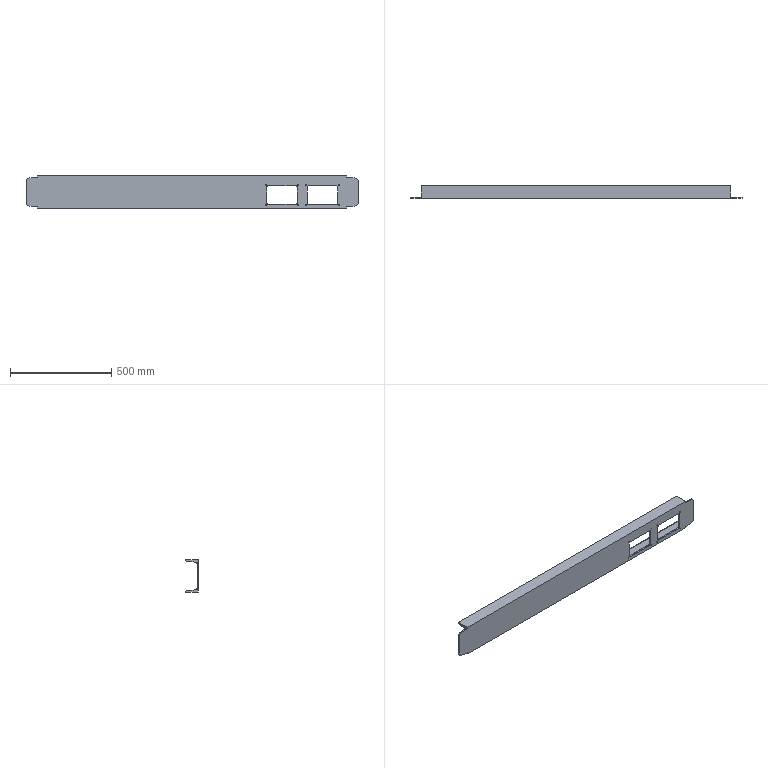Part | SolidWorks | 1 solid | 62 faces | box 1637 x 63 x 160 mm | volume 3270574 mm3 | plane 34 | cylinder 28 | commonest cylinder face diameters 5 x16 10 x10 20 x2